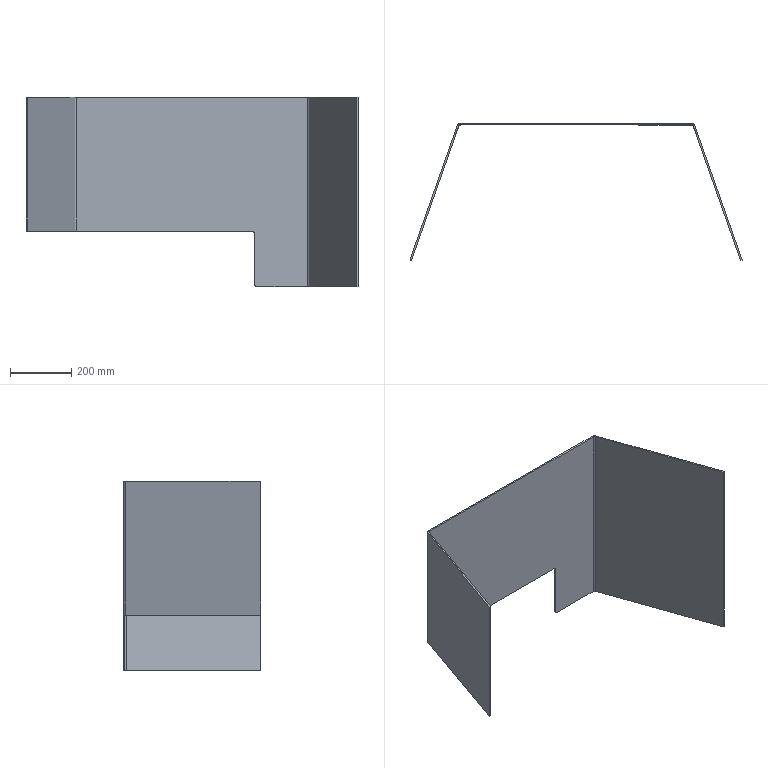Part | SolidWorks | features Fillet 2, Cut 1, FlatPattern 1, SMBaseFlange 1, SheetMetal 1, UnFold 1 | 1 solid | 24 faces | box 1088 x 449.658 x 620 mm | volume 4342657 mm3 | plane 18 | cylinder 6 | commonest cylinder face diameters 12 x2 22 x2 14 x1 20 x1
STEP:
#1=CARTESIAN_POINT('',(-378.607,0.,620.));
#2=VERTEX_POINT('',#1);
#3=CARTESIAN_POINT('',(-378.607,-5.,620.));
#4=VERTEX_POINT('',#3);
#5=CARTESIAN_POINT('',(-378.607,0.,620.));
#6=DIRECTION('',(0.,-1.,0.));
#7=VECTOR('',#6,1000.);
#8=LINE('',#5,#7);
#9=EDGE_CURVE('',#2,#4,#8,.T.);
#10=ORIENTED_EDGE('',*,*,#9,.F.);
#11=CARTESIAN_POINT('',(-388.985,-7.352,620.));
#12=VERTEX_POINT('',#11);
#13=CARTESIAN_POINT('',(-378.607,-11.,620.));
#14=DIRECTION('',(0.,0.,1.));
#15=DIRECTION('',(1.,0.,0.));
#16=AXIS2_PLACEMENT_3D('',#13,#14,#15);
#17=CIRCLE('',#16,11.);
#18=EDGE_CURVE('',#2,#12,#17,.T.);
#19=ORIENTED_EDGE('',*,*,#18,.T.);
#20=CARTESIAN_POINT('',(-384.268,-9.01,620.));
#21=VERTEX_POINT('',#20);
#22=CARTESIAN_POINT('',(-384.268,-9.01,620.));
#23=DIRECTION('',(-0.9434,0.3317,0.));
#24=VECTOR('',#23,1000.);
#25=LINE('',#22,#24);
#26=EDGE_CURVE('',#21,#12,#25,.T.);
#27=ORIENTED_EDGE('',*,*,#26,.F.);
#28=CARTESIAN_POINT('',(-378.607,-11.,620.));
#29=DIRECTION('',(0.,0.,1.));
#30=DIRECTION('',(1.,0.,0.));
#31=AXIS2_PLACEMENT_3D('',#28,#29,#30);
#32=CIRCLE('',#31,6.);
#33=EDGE_CURVE('',#4,#21,#32,.T.);
#34=ORIENTED_EDGE('',*,*,#33,.F.);
#35=EDGE_LOOP('',(#10,#19,#27,#34));
#36=FACE_OUTER_BOUND('',#35,.T.);
#37=CARTESIAN_POINT('',(-378.607,0.,620.));
#38=DIRECTION('',(0.,0.,1.));
#39=DIRECTION('',(1.,0.,0.));
#40=AXIS2_PLACEMENT_3D('',#37,#38,#39);
#41=PLANE('',#40);
#42=ADVANCED_FACE('',(#36),#41,.T.);
#43=CARTESIAN_POINT('',(378.607,0.,620.));
#44=VERTEX_POINT('',#43);
#45=CARTESIAN_POINT('',(-386.4,0.,620.));
#46=DIRECTION('',(-1.,0.,0.));
#47=VECTOR('',#46,1000.);
#48=LINE('',#45,#47);
#49=EDGE_CURVE('',#44,#2,#48,.T.);
#50=ORIENTED_EDGE('',*,*,#49,.T.);
#51=ORIENTED_EDGE('',*,*,#9,.T.);
#52=CARTESIAN_POINT('',(378.607,-5.,620.));
#53=VERTEX_POINT('',#52);
#54=CARTESIAN_POINT('',(-386.4,-5.,620.));
#55=DIRECTION('',(-1.,0.,0.));
#56=VECTOR('',#55,1000.);
#57=LINE('',#54,#56);
#58=EDGE_CURVE('',#53,#4,#57,.T.);
#59=ORIENTED_EDGE('',*,*,#58,.F.);
#60=CARTESIAN_POINT('',(378.607,-5.,620.));
#61=DIRECTION('',(0.,1.,0.));
#62=VECTOR('',#61,1000.);
#63=LINE('',#60,#62);
#64=EDGE_CURVE('',#53,#44,#63,.T.);
#65=ORIENTED_EDGE('',*,*,#64,.T.);
#66=EDGE_LOOP('',(#50,#51,#59,#65));
#67=FACE_OUTER_BOUND('',#66,.T.);
#68=CARTESIAN_POINT('',(-384.268,-9.01,620.));
#69=DIRECTION('',(0.,0.,1.));
#70=DIRECTION('',(1.,0.,0.));
#71=AXIS2_PLACEMENT_3D('',#68,#69,#70);
#72=PLANE('',#71);
#73=ADVANCED_FACE('',(#67),#72,.T.);
#74=CARTESIAN_POINT('',(388.985,-7.352,620.));
#75=VERTEX_POINT('',#74);
#76=CARTESIAN_POINT('',(384.268,-9.01,620.));
#77=VERTEX_POINT('',#76);
#78=CARTESIAN_POINT('',(388.985,-7.352,620.));
#79=DIRECTION('',(-0.9434,-0.3317,0.));
#80=VECTOR('',#79,1000.);
#81=LINE('',#78,#80);
#82=EDGE_CURVE('',#75,#77,#81,.T.);
#83=ORIENTED_EDGE('',*,*,#82,.F.);
#84=CARTESIAN_POINT('',(378.607,-11.,620.));
#85=DIRECTION('',(0.,0.,1.));
#86=DIRECTION('',(1.,0.,0.));
#87=AXIS2_PLACEMENT_3D('',#84,#85,#86);
#88=CIRCLE('',#87,11.);
#89=EDGE_CURVE('',#75,#44,#88,.T.);
#90=ORIENTED_EDGE('',*,*,#89,.T.);
#91=ORIENTED_EDGE('',*,*,#64,.F.);
#92=CARTESIAN_POINT('',(378.607,-11.,620.));
#93=DIRECTION('',(0.,0.,1.));
#94=DIRECTION('',(1.,0.,0.));
#95=AXIS2_PLACEMENT_3D('',#92,#93,#94);
#96=CIRCLE('',#95,6.);
#97=EDGE_CURVE('',#77,#53,#96,.T.);
#98=ORIENTED_EDGE('',*,*,#97,.F.);
#99=EDGE_LOOP('',(#83,#90,#91,#98));
#100=FACE_OUTER_BOUND('',#99,.T.);
#101=CARTESIAN_POINT('',(388.985,-7.352,620.));
#102=DIRECTION('',(0.,0.,1.));
#103=DIRECTION('',(1.,0.,0.));
#104=AXIS2_PLACEMENT_3D('',#101,#102,#103);
#105=PLANE('',#104);
#106=ADVANCED_FACE('',(#100),#105,.T.);
#107=CARTESIAN_POINT('',(543.902,-448.,620.));
#108=VERTEX_POINT('',#107);
#109=CARTESIAN_POINT('',(543.902,-448.,620.));
#110=DIRECTION('',(-0.3317,0.9434,0.));
#111=VECTOR('',#110,1000.);
#112=LINE('',#109,#111);
#113=EDGE_CURVE('',#108,#75,#112,.T.);
#114=ORIENTED_EDGE('',*,*,#113,.T.);
#115=ORIENTED_EDGE('',*,*,#82,.T.);
#116=CARTESIAN_POINT('',(539.185,-449.658,620.));
#117=VERTEX_POINT('',#116);
#118=CARTESIAN_POINT('',(539.185,-449.658,620.));
#119=DIRECTION('',(-0.3317,0.9434,0.));
#120=VECTOR('',#119,1000.);
#121=LINE('',#118,#120);
#122=EDGE_CURVE('',#117,#77,#121,.T.);
#123=ORIENTED_EDGE('',*,*,#122,.F.);
#124=CARTESIAN_POINT('',(543.902,-448.,620.));
#125=DIRECTION('',(-0.9434,-0.3317,0.));
#126=VECTOR('',#125,1000.);
#127=LINE('',#124,#126);
#128=EDGE_CURVE('',#108,#117,#127,.T.);
#129=ORIENTED_EDGE('',*,*,#128,.F.);
#130=EDGE_LOOP('',(#114,#115,#123,#129));
#131=FACE_OUTER_BOUND('',#130,.T.);
#132=CARTESIAN_POINT('',(378.607,-5.,620.));
#133=DIRECTION('',(0.,0.,1.));
#134=DIRECTION('',(1.,0.,0.));
#135=AXIS2_PLACEMENT_3D('',#132,#133,#134);
#136=PLANE('',#135);
#137=ADVANCED_FACE('',(#131),#136,.T.);
#138=CARTESIAN_POINT('',(378.607,0.,0.));
#139=VERTEX_POINT('',#138);
#140=CARTESIAN_POINT('',(378.607,-5.,0.));
#141=VERTEX_POINT('',#140);
#142=CARTESIAN_POINT('',(378.607,0.,0.));
#143=DIRECTION('',(0.,-1.,0.));
#144=VECTOR('',#143,1000.);
#145=LINE('',#142,#144);
#146=EDGE_CURVE('',#139,#141,#145,.T.);
#147=ORIENTED_EDGE('',*,*,#146,.F.);
#148=CARTESIAN_POINT('',(388.985,-7.352,0.));
#149=VERTEX_POINT('',#148);
#150=CARTESIAN_POINT('',(378.607,-11.,0.));
#151=DIRECTION('',(0.,0.,1.));
#152=DIRECTION('',(1.,0.,0.));
#153=AXIS2_PLACEMENT_3D('',#150,#151,#152);
#154=CIRCLE('',#153,11.);
#155=EDGE_CURVE('',#149,#139,#154,.T.);
#156=ORIENTED_EDGE('',*,*,#155,.F.);
#157=CARTESIAN_POINT('',(384.268,-9.01,0.));
#158=VERTEX_POINT('',#157);
#159=CARTESIAN_POINT('',(384.268,-9.01,0.));
#160=DIRECTION('',(0.9434,0.3317,0.));
#161=VECTOR('',#160,1000.);
#162=LINE('',#159,#161);
#163=EDGE_CURVE('',#158,#149,#162,.T.);
#164=ORIENTED_EDGE('',*,*,#163,.F.);
#165=CARTESIAN_POINT('',(378.607,-11.,0.));
#166=DIRECTION('',(0.,0.,1.));
#167=DIRECTION('',(1.,0.,0.));
#168=AXIS2_PLACEMENT_3D('',#165,#166,#167);
#169=CIRCLE('',#168,6.);
#170=EDGE_CURVE('',#158,#141,#169,.T.);
#171=ORIENTED_EDGE('',*,*,#170,.T.);
#172=EDGE_LOOP('',(#147,#156,#164,#171));
#173=FACE_OUTER_BOUND('',#172,.T.);
#174=CARTESIAN_POINT('',(378.607,0.,0.));
#175=DIRECTION('',(0.,0.,-1.));
#176=DIRECTION('',(-1.,0.,0.));
#177=AXIS2_PLACEMENT_3D('',#174,#175,#176);
#178=PLANE('',#177);
#179=ADVANCED_FACE('',(#173),#178,.T.);
#180=CARTESIAN_POINT('',(212.,-5.,0.));
#181=VERTEX_POINT('',#180);
#182=CARTESIAN_POINT('',(-386.4,-5.,0.));
#183=DIRECTION('',(-1.,0.,0.));
#184=VECTOR('',#183,1000.);
#185=LINE('',#182,#184);
#186=EDGE_CURVE('',#141,#181,#185,.T.);
#187=ORIENTED_EDGE('',*,*,#186,.T.);
#188=CARTESIAN_POINT('',(212.,0.,0.));
#189=VERTEX_POINT('',#188);
#190=CARTESIAN_POINT('',(212.,0.,0.));
#191=DIRECTION('',(0.,1.,0.));
#192=VECTOR('',#191,1000.);
#193=LINE('',#190,#192);
#194=EDGE_CURVE('',#181,#189,#193,.T.);
#195=ORIENTED_EDGE('',*,*,#194,.T.);
#196=CARTESIAN_POINT('',(-386.4,0.,0.));
#197=DIRECTION('',(-1.,0.,0.));
#198=VECTOR('',#197,1000.);
#199=LINE('',#196,#198);
#200=EDGE_CURVE('',#139,#189,#199,.T.);
#201=ORIENTED_EDGE('',*,*,#200,.F.);
#202=ORIENTED_EDGE('',*,*,#146,.T.);
#203=EDGE_LOOP('',(#187,#195,#201,#202));
#204=FACE_OUTER_BOUND('',#203,.T.);
#205=CARTESIAN_POINT('',(384.268,-9.01,0.));
#206=DIRECTION('',(0.,0.,-1.));
#207=DIRECTION('',(-1.,0.,0.));
#208=AXIS2_PLACEMENT_3D('',#205,#206,#207);
#209=PLANE('',#208);
#210=ADVANCED_FACE('',(#204),#209,.T.);
#211=CARTESIAN_POINT('',(-388.985,-7.352,182.));
#212=VERTEX_POINT('',#211);
#213=CARTESIAN_POINT('',(-388.985,-7.352,620.));
#214=DIRECTION('',(0.,0.,-1.));
#215=VECTOR('',#214,1000.);
#216=LINE('',#213,#215);
#217=EDGE_CURVE('',#12,#212,#216,.T.);
#218=ORIENTED_EDGE('',*,*,#217,.T.);
#219=CARTESIAN_POINT('',(-543.902,-448.,182.));
#220=VERTEX_POINT('',#219);
#221=CARTESIAN_POINT('',(-543.902,-448.,182.));
#222=DIRECTION('',(-0.3317,-0.9434,0.));
#223=VECTOR('',#222,1000.);
#224=LINE('',#221,#223);
#225=EDGE_CURVE('',#212,#220,#224,.T.);
#226=ORIENTED_EDGE('',*,*,#225,.T.);
#227=CARTESIAN_POINT('',(-543.902,-448.,620.));
#228=VERTEX_POINT('',#227);
#229=CARTESIAN_POINT('',(-543.902,-448.,620.));
#230=DIRECTION('',(0.,0.,-1.));
#231=VECTOR('',#230,1000.);
#232=LINE('',#229,#231);
#233=EDGE_CURVE('',#228,#220,#232,.T.);
#234=ORIENTED_EDGE('',*,*,#233,.F.);
#235=CARTESIAN_POINT('',(-543.902,-448.,620.));
#236=DIRECTION('',(-0.3317,-0.9434,0.));
#237=VECTOR('',#236,1000.);
#238=LINE('',#235,#237);
#239=EDGE_CURVE('',#12,#228,#238,.T.);
#240=ORIENTED_EDGE('',*,*,#239,.F.);
#241=EDGE_LOOP('',(#218,#226,#234,#240));
#242=FACE_OUTER_BOUND('',#241,.T.);
#243=CARTESIAN_POINT('',(-543.902,-448.,620.));
#244=DIRECTION('',(0.9434,-0.3317,0.));
#245=DIRECTION('',(0.3317,0.9434,0.));
#246=AXIS2_PLACEMENT_3D('',#243,#244,#245);
#247=PLANE('',#246);
#248=ADVANCED_FACE('',(#242),#247,.F.);
#249=CARTESIAN_POINT('',(-539.185,-449.658,182.));
#250=VERTEX_POINT('',#249);
#251=CARTESIAN_POINT('',(-539.185,-449.658,182.));
#252=DIRECTION('',(-0.9434,0.3317,0.));
#253=VECTOR('',#252,1000.);
#254=LINE('',#251,#253);
#255=EDGE_CURVE('',#250,#220,#254,.T.);
#256=ORIENTED_EDGE('',*,*,#255,.F.);
#257=CARTESIAN_POINT('',(-539.185,-449.658,620.));
#258=VERTEX_POINT('',#257);
#259=CARTESIAN_POINT('',(-539.185,-449.658,620.));
#260=DIRECTION('',(0.,0.,-1.));
#261=VECTOR('',#260,1000.);
#262=LINE('',#259,#261);
#263=EDGE_CURVE('',#258,#250,#262,.T.);
#264=ORIENTED_EDGE('',*,*,#263,.F.);
#265=CARTESIAN_POINT('',(-539.185,-449.658,620.));
#266=DIRECTION('',(-0.9434,0.3317,0.));
#267=VECTOR('',#266,1000.);
#268=LINE('',#265,#267);
#269=EDGE_CURVE('',#258,#228,#268,.T.);
#270=ORIENTED_EDGE('',*,*,#269,.T.);
#271=ORIENTED_EDGE('',*,*,#233,.T.);
#272=EDGE_LOOP('',(#256,#264,#270,#271));
#273=FACE_OUTER_BOUND('',#272,.T.);
#274=CARTESIAN_POINT('',(-539.185,-449.658,620.));
#275=DIRECTION('',(-0.3317,-0.9434,0.));
#276=DIRECTION('',(0.9434,-0.3317,0.));
#277=AXIS2_PLACEMENT_3D('',#274,#275,#276);
#278=PLANE('',#277);
#279=ADVANCED_FACE('',(#273),#278,.T.);
#280=CARTESIAN_POINT('',(-384.268,-9.01,182.));
#281=VERTEX_POINT('',#280);
#282=CARTESIAN_POINT('',(-539.185,-449.658,182.));
#283=DIRECTION('',(-0.3317,-0.9434,0.));
#284=VECTOR('',#283,1000.);
#285=LINE('',#282,#284);
#286=EDGE_CURVE('',#281,#250,#285,.T.);
#287=ORIENTED_EDGE('',*,*,#286,.F.);
#288=CARTESIAN_POINT('',(-384.268,-9.01,620.));
#289=DIRECTION('',(0.,0.,-1.));
#290=VECTOR('',#289,1000.);
#291=LINE('',#288,#290);
#292=EDGE_CURVE('',#21,#281,#291,.T.);
#293=ORIENTED_EDGE('',*,*,#292,.F.);
#294=CARTESIAN_POINT('',(-539.185,-449.658,620.));
#295=DIRECTION('',(-0.3317,-0.9434,0.));
#296=VECTOR('',#295,1000.);
#297=LINE('',#294,#296);
#298=EDGE_CURVE('',#21,#258,#297,.T.);
#299=ORIENTED_EDGE('',*,*,#298,.T.);
#300=ORIENTED_EDGE('',*,*,#263,.T.);
#301=EDGE_LOOP('',(#287,#293,#299,#300));
#302=FACE_OUTER_BOUND('',#301,.T.);
#303=CARTESIAN_POINT('',(-539.185,-449.658,620.));
#304=DIRECTION('',(0.9434,-0.3317,0.));
#305=DIRECTION('',(0.3317,0.9434,0.));
#306=AXIS2_PLACEMENT_3D('',#303,#304,#305);
#307=PLANE('',#306);
#308=ADVANCED_FACE('',(#302),#307,.T.);
#309=CARTESIAN_POINT('',(-378.607,-5.,182.));
#310=VERTEX_POINT('',#309);
#311=CARTESIAN_POINT('',(-378.607,-11.,182.));
#312=DIRECTION('',(0.,0.,1.));
#313=DIRECTION('',(1.,0.,0.));
#314=AXIS2_PLACEMENT_3D('',#311,#312,#313);
#315=CIRCLE('',#314,6.);
#316=EDGE_CURVE('',#310,#281,#315,.T.);
#317=ORIENTED_EDGE('',*,*,#316,.F.);
#318=CARTESIAN_POINT('',(-378.607,-5.,620.));
#319=DIRECTION('',(0.,0.,-1.));
#320=VECTOR('',#319,1000.);
#321=LINE('',#318,#320);
#322=EDGE_CURVE('',#4,#310,#321,.T.);
#323=ORIENTED_EDGE('',*,*,#322,.F.);
#324=ORIENTED_EDGE('',*,*,#33,.T.);
#325=ORIENTED_EDGE('',*,*,#292,.T.);
#326=EDGE_LOOP('',(#317,#323,#324,#325));
#327=FACE_OUTER_BOUND('',#326,.T.);
#328=CARTESIAN_POINT('',(-378.607,-11.,620.));
#329=DIRECTION('',(0.,0.,-1.));
#330=DIRECTION('',(-1.,0.,0.));
#331=AXIS2_PLACEMENT_3D('',#328,#329,#330);
#332=CYLINDRICAL_SURFACE('',#331,6.);
#333=ADVANCED_FACE('',(#327),#332,.F.);
#334=CARTESIAN_POINT('',(205.,-5.,7.));
#335=VERTEX_POINT('',#334);
#336=CARTESIAN_POINT('',(205.,-5.,172.));
#337=VERTEX_POINT('',#336);
#338=CARTESIAN_POINT('',(205.,-5.,620.));
#339=DIRECTION('',(0.,0.,1.));
#340=VECTOR('',#339,1000.);
#341=LINE('',#338,#340);
#342=EDGE_CURVE('',#335,#337,#341,.T.);
#343=ORIENTED_EDGE('',*,*,#342,.F.);
#344=CARTESIAN_POINT('',(212.,-5.,7.));
#345=DIRECTION('',(0.,-1.,0.));
#346=DIRECTION('',(1.,0.,0.));
#347=AXIS2_PLACEMENT_3D('',#344,#345,#346);
#348=CIRCLE('',#347,7.);
#349=EDGE_CURVE('',#335,#181,#348,.T.);
#350=ORIENTED_EDGE('',*,*,#349,.T.);
#351=ORIENTED_EDGE('',*,*,#186,.F.);
#352=CARTESIAN_POINT('',(378.607,-5.,620.));
#353=DIRECTION('',(0.,0.,-1.));
#354=VECTOR('',#353,1000.);
#355=LINE('',#352,#354);
#356=EDGE_CURVE('',#53,#141,#355,.T.);
#357=ORIENTED_EDGE('',*,*,#356,.F.);
#358=ORIENTED_EDGE('',*,*,#58,.T.);
#359=ORIENTED_EDGE('',*,*,#322,.T.);
#360=CARTESIAN_POINT('',(195.,-5.,182.));
#361=VERTEX_POINT('',#360);
#362=CARTESIAN_POINT('',(-386.4,-5.,182.));
#363=DIRECTION('',(-1.,0.,0.));
#364=VECTOR('',#363,1000.);
#365=LINE('',#362,#364);
#366=EDGE_CURVE('',#361,#310,#365,.T.);
#367=ORIENTED_EDGE('',*,*,#366,.F.);
#368=CARTESIAN_POINT('',(195.,-5.,172.));
#369=DIRECTION('',(0.,1.,0.));
#370=DIRECTION('',(1.,0.,0.));
#371=AXIS2_PLACEMENT_3D('',#368,#369,#370);
#372=CIRCLE('',#371,10.);
#373=EDGE_CURVE('',#361,#337,#372,.T.);
#374=ORIENTED_EDGE('',*,*,#373,.T.);
#375=EDGE_LOOP('',(#343,#350,#351,#357,#358,#359,#367,#374));
#376=FACE_OUTER_BOUND('',#375,.T.);
#377=CARTESIAN_POINT('',(-386.4,-5.,620.));
#378=DIRECTION('',(0.,-1.,0.));
#379=DIRECTION('',(1.,0.,0.));
#380=AXIS2_PLACEMENT_3D('',#377,#378,#379);
#381=PLANE('',#380);
#382=ADVANCED_FACE('',(#376),#381,.T.);
#383=ORIENTED_EDGE('',*,*,#170,.F.);
#384=CARTESIAN_POINT('',(384.268,-9.01,620.));
#385=DIRECTION('',(0.,0.,-1.));
#386=VECTOR('',#385,1000.);
#387=LINE('',#384,#386);
#388=EDGE_CURVE('',#77,#158,#387,.T.);
#389=ORIENTED_EDGE('',*,*,#388,.F.);
#390=ORIENTED_EDGE('',*,*,#97,.T.);
#391=ORIENTED_EDGE('',*,*,#356,.T.);
#392=EDGE_LOOP('',(#383,#389,#390,#391));
#393=FACE_OUTER_BOUND('',#392,.T.);
#394=CARTESIAN_POINT('',(378.607,-11.,620.));
#395=DIRECTION('',(0.,0.,-1.));
#396=DIRECTION('',(-1.,0.,0.));
#397=AXIS2_PLACEMENT_3D('',#394,#395,#396);
#398=CYLINDRICAL_SURFACE('',#397,6.);
#399=ADVANCED_FACE('',(#393),#398,.F.);
#400=CARTESIAN_POINT('',(539.185,-449.658,0.));
#401=VERTEX_POINT('',#400);
#402=CARTESIAN_POINT('',(539.185,-449.658,0.));
#403=DIRECTION('',(-0.3317,0.9434,0.));
#404=VECTOR('',#403,1000.);
#405=LINE('',#402,#404);
#406=EDGE_CURVE('',#401,#158,#405,.T.);
#407=ORIENTED_EDGE('',*,*,#406,.F.);
#408=CARTESIAN_POINT('',(539.185,-449.658,620.));
#409=DIRECTION('',(0.,0.,-1.));
#410=VECTOR('',#409,1000.);
#411=LINE('',#408,#410);
#412=EDGE_CURVE('',#117,#401,#411,.T.);
#413=ORIENTED_EDGE('',*,*,#412,.F.);
#414=ORIENTED_EDGE('',*,*,#122,.T.);
#415=ORIENTED_EDGE('',*,*,#388,.T.);
#416=EDGE_LOOP('',(#407,#413,#414,#415));
#417=FACE_OUTER_BOUND('',#416,.T.);
#418=CARTESIAN_POINT('',(539.185,-449.658,620.));
#419=DIRECTION('',(-0.9434,-0.3317,0.));
#420=DIRECTION('',(0.3317,-0.9434,0.));
#421=AXIS2_PLACEMENT_3D('',#418,#419,#420);
#422=PLANE('',#421);
#423=ADVANCED_FACE('',(#417),#422,.T.);
#424=CARTESIAN_POINT('',(543.902,-448.,0.));
#425=VERTEX_POINT('',#424);
#426=CARTESIAN_POINT('',(543.902,-448.,0.));
#427=DIRECTION('',(-0.9434,-0.3317,0.));
#428=VECTOR('',#427,1000.);
#429=LINE('',#426,#428);
#430=EDGE_CURVE('',#425,#401,#429,.T.);
#431=ORIENTED_EDGE('',*,*,#430,.F.);
#432=CARTESIAN_POINT('',(543.902,-448.,620.));
#433=DIRECTION('',(0.,0.,-1.));
#434=VECTOR('',#433,1000.);
#435=LINE('',#432,#434);
#436=EDGE_CURVE('',#108,#425,#435,.T.);
#437=ORIENTED_EDGE('',*,*,#436,.F.);
#438=ORIENTED_EDGE('',*,*,#128,.T.);
#439=ORIENTED_EDGE('',*,*,#412,.T.);
#440=EDGE_LOOP('',(#431,#437,#438,#439));
#441=FACE_OUTER_BOUND('',#440,.T.);
#442=CARTESIAN_POINT('',(543.902,-448.,620.));
#443=DIRECTION('',(0.3317,-0.9434,0.));
#444=DIRECTION('',(0.9434,0.3317,0.));
#445=AXIS2_PLACEMENT_3D('',#442,#443,#444);
#446=PLANE('',#445);
#447=ADVANCED_FACE('',(#441),#446,.T.);
#448=CARTESIAN_POINT('',(543.902,-448.,0.));
#449=DIRECTION('',(-0.3317,0.9434,0.));
#450=VECTOR('',#449,1000.);
#451=LINE('',#448,#450);
#452=EDGE_CURVE('',#425,#149,#451,.T.);
#453=ORIENTED_EDGE('',*,*,#452,.T.);
#454=CARTESIAN_POINT('',(388.985,-7.352,620.));
#455=DIRECTION('',(0.,0.,-1.));
#456=VECTOR('',#455,1000.);
#457=LINE('',#454,#456);
#458=EDGE_CURVE('',#75,#149,#457,.T.);
#459=ORIENTED_EDGE('',*,*,#458,.F.);
#460=ORIENTED_EDGE('',*,*,#113,.F.);
#461=ORIENTED_EDGE('',*,*,#436,.T.);
#462=EDGE_LOOP('',(#453,#459,#460,#461));
#463=FACE_OUTER_BOUND('',#462,.T.);
#464=CARTESIAN_POINT('',(543.902,-448.,620.));
#465=DIRECTION('',(-0.9434,-0.3317,0.));
#466=DIRECTION('',(0.3317,-0.9434,0.));
#467=AXIS2_PLACEMENT_3D('',#464,#465,#466);
#468=PLANE('',#467);
#469=ADVANCED_FACE('',(#463),#468,.F.);
#470=ORIENTED_EDGE('',*,*,#155,.T.);
#471=CARTESIAN_POINT('',(378.607,0.,620.));
#472=DIRECTION('',(0.,0.,-1.));
#473=VECTOR('',#472,1000.);
#474=LINE('',#471,#473);
#475=EDGE_CURVE('',#44,#139,#474,.T.);
#476=ORIENTED_EDGE('',*,*,#475,.F.);
#477=ORIENTED_EDGE('',*,*,#89,.F.);
#478=ORIENTED_EDGE('',*,*,#458,.T.);
#479=EDGE_LOOP('',(#470,#476,#477,#478));
#480=FACE_OUTER_BOUND('',#479,.T.);
#481=CARTESIAN_POINT('',(378.607,-11.,620.));
#482=DIRECTION('',(0.,0.,-1.));
#483=DIRECTION('',(-1.,0.,0.));
#484=AXIS2_PLACEMENT_3D('',#481,#482,#483);
#485=CYLINDRICAL_SURFACE('',#484,11.);
#486=ADVANCED_FACE('',(#480),#485,.T.);
#487=ORIENTED_EDGE('',*,*,#200,.T.);
#488=CARTESIAN_POINT('',(205.,0.,7.));
#489=VERTEX_POINT('',#488);
#490=CARTESIAN_POINT('',(212.,0.,7.));
#491=DIRECTION('',(0.,1.,0.));
#492=DIRECTION('',(1.,0.,0.));
#493=AXIS2_PLACEMENT_3D('',#490,#491,#492);
#494=CIRCLE('',#493,7.);
#495=EDGE_CURVE('',#189,#489,#494,.T.);
#496=ORIENTED_EDGE('',*,*,#495,.T.);
#497=CARTESIAN_POINT('',(205.,0.,172.));
#498=VERTEX_POINT('',#497);
#499=CARTESIAN_POINT('',(205.,0.,620.));
#500=DIRECTION('',(0.,0.,1.));
#501=VECTOR('',#500,1000.);
#502=LINE('',#499,#501);
#503=EDGE_CURVE('',#489,#498,#502,.T.);
#504=ORIENTED_EDGE('',*,*,#503,.T.);
#505=CARTESIAN_POINT('',(195.,0.,182.));
#506=VERTEX_POINT('',#505);
#507=CARTESIAN_POINT('',(195.,0.,172.));
#508=DIRECTION('',(0.,-1.,0.));
#509=DIRECTION('',(1.,0.,0.));
#510=AXIS2_PLACEMENT_3D('',#507,#508,#509);
#511=CIRCLE('',#510,10.);
#512=EDGE_CURVE('',#498,#506,#511,.T.);
#513=ORIENTED_EDGE('',*,*,#512,.T.);
#514=CARTESIAN_POINT('',(-378.607,0.,182.));
#515=VERTEX_POINT('',#514);
#516=CARTESIAN_POINT('',(-386.4,0.,182.));
#517=DIRECTION('',(-1.,0.,0.));
#518=VECTOR('',#517,1000.);
#519=LINE('',#516,#518);
#520=EDGE_CURVE('',#506,#515,#519,.T.);
#521=ORIENTED_EDGE('',*,*,#520,.T.);
#522=CARTESIAN_POINT('',(-378.607,0.,620.));
#523=DIRECTION('',(0.,0.,-1.));
#524=VECTOR('',#523,1000.);
#525=LINE('',#522,#524);
#526=EDGE_CURVE('',#2,#515,#525,.T.);
#527=ORIENTED_EDGE('',*,*,#526,.F.);
#528=ORIENTED_EDGE('',*,*,#49,.F.);
#529=ORIENTED_EDGE('',*,*,#475,.T.);
#530=EDGE_LOOP('',(#487,#496,#504,#513,#521,#527,#528,#529));
#531=FACE_OUTER_BOUND('',#530,.T.);
#532=CARTESIAN_POINT('',(-386.4,0.,620.));
#533=DIRECTION('',(0.,-1.,0.));
#534=DIRECTION('',(1.,0.,0.));
#535=AXIS2_PLACEMENT_3D('',#532,#533,#534);
#536=PLANE('',#535);
#537=ADVANCED_FACE('',(#531),#536,.F.);
#538=ORIENTED_EDGE('',*,*,#526,.T.);
#539=CARTESIAN_POINT('',(-378.607,-11.,182.));
#540=DIRECTION('',(0.,0.,1.));
#541=DIRECTION('',(1.,0.,0.));
#542=AXIS2_PLACEMENT_3D('',#539,#540,#541);
#543=CIRCLE('',#542,11.);
#544=EDGE_CURVE('',#515,#212,#543,.T.);
#545=ORIENTED_EDGE('',*,*,#544,.T.);
#546=ORIENTED_EDGE('',*,*,#217,.F.);
#547=ORIENTED_EDGE('',*,*,#18,.F.);
#548=EDGE_LOOP('',(#538,#545,#546,#547));
#549=FACE_OUTER_BOUND('',#548,.T.);
#550=CARTESIAN_POINT('',(-378.607,-11.,620.));
#551=DIRECTION('',(0.,0.,-1.));
#552=DIRECTION('',(-1.,0.,0.));
#553=AXIS2_PLACEMENT_3D('',#550,#551,#552);
#554=CYLINDRICAL_SURFACE('',#553,11.);
#555=ADVANCED_FACE('',(#549),#554,.T.);
#556=ORIENTED_EDGE('',*,*,#239,.T.);
#557=ORIENTED_EDGE('',*,*,#269,.F.);
#558=ORIENTED_EDGE('',*,*,#298,.F.);
#559=ORIENTED_EDGE('',*,*,#26,.T.);
#560=EDGE_LOOP('',(#556,#557,#558,#559));
#561=FACE_OUTER_BOUND('',#560,.T.);
#562=CARTESIAN_POINT('',(-378.607,-11.,620.));
#563=DIRECTION('',(0.,0.,1.));
#564=DIRECTION('',(1.,0.,0.));
#565=AXIS2_PLACEMENT_3D('',#562,#563,#564);
#566=PLANE('',#565);
#567=ADVANCED_FACE('',(#561),#566,.T.);
#568=ORIENTED_EDGE('',*,*,#406,.T.);
#569=ORIENTED_EDGE('',*,*,#163,.T.);
#570=ORIENTED_EDGE('',*,*,#452,.F.);
#571=ORIENTED_EDGE('',*,*,#430,.T.);
#572=EDGE_LOOP('',(#568,#569,#570,#571));
#573=FACE_OUTER_BOUND('',#572,.T.);
#574=CARTESIAN_POINT('',(-378.607,-11.,0.));
#575=DIRECTION('',(0.,0.,1.));
#576=DIRECTION('',(1.,0.,0.));
#577=AXIS2_PLACEMENT_3D('',#574,#575,#576);
#578=PLANE('',#577);
#579=ADVANCED_FACE('',(#573),#578,.F.);
#580=ORIENTED_EDGE('',*,*,#342,.T.);
#581=CARTESIAN_POINT('',(205.,0.,172.));
#582=DIRECTION('',(0.,1.,0.));
#583=VECTOR('',#582,1000.);
#584=LINE('',#581,#583);
#585=EDGE_CURVE('',#337,#498,#584,.T.);
#586=ORIENTED_EDGE('',*,*,#585,.T.);
#587=ORIENTED_EDGE('',*,*,#503,.F.);
#588=CARTESIAN_POINT('',(205.,-5.,7.));
#589=DIRECTION('',(0.,-1.,0.));
#590=VECTOR('',#589,1000.);
#591=LINE('',#588,#590);
#592=EDGE_CURVE('',#489,#335,#591,.T.);
#593=ORIENTED_EDGE('',*,*,#592,.T.);
#594=EDGE_LOOP('',(#580,#586,#587,#593));
#595=FACE_OUTER_BOUND('',#594,.T.);
#596=CARTESIAN_POINT('',(205.,-449.658,-60.503));
#597=DIRECTION('',(1.,0.,0.));
#598=DIRECTION('',(0.,0.,-1.));
#599=AXIS2_PLACEMENT_3D('',#596,#597,#598);
#600=PLANE('',#599);
#601=ADVANCED_FACE('',(#595),#600,.F.);
#602=ORIENTED_EDGE('',*,*,#520,.F.);
#603=CARTESIAN_POINT('',(195.,-5.,182.));
#604=DIRECTION('',(0.,-1.,0.));
#605=VECTOR('',#604,1000.);
#606=LINE('',#603,#605);
#607=EDGE_CURVE('',#506,#361,#606,.T.);
#608=ORIENTED_EDGE('',*,*,#607,.T.);
#609=ORIENTED_EDGE('',*,*,#366,.T.);
#610=ORIENTED_EDGE('',*,*,#316,.T.);
#611=ORIENTED_EDGE('',*,*,#286,.T.);
#612=ORIENTED_EDGE('',*,*,#255,.T.);
#613=ORIENTED_EDGE('',*,*,#225,.F.);
#614=ORIENTED_EDGE('',*,*,#544,.F.);
#615=EDGE_LOOP('',(#602,#608,#609,#610,#611,#612,#613,#614));
#616=FACE_OUTER_BOUND('',#615,.T.);
#617=CARTESIAN_POINT('',(-661.016,-449.658,182.));
#618=DIRECTION('',(0.,0.,1.));
#619=DIRECTION('',(1.,0.,0.));
#620=AXIS2_PLACEMENT_3D('',#617,#618,#619);
#621=PLANE('',#620);
#622=ADVANCED_FACE('',(#616),#621,.F.);
#623=ORIENTED_EDGE('',*,*,#495,.F.);
#624=ORIENTED_EDGE('',*,*,#194,.F.);
#625=ORIENTED_EDGE('',*,*,#349,.F.);
#626=ORIENTED_EDGE('',*,*,#592,.F.);
#627=EDGE_LOOP('',(#623,#624,#625,#626));
#628=FACE_OUTER_BOUND('',#627,.T.);
#629=CARTESIAN_POINT('',(212.,-449.658,7.));
#630=DIRECTION('',(0.,1.,0.));
#631=DIRECTION('',(0.,0.,1.));
#632=AXIS2_PLACEMENT_3D('',#629,#630,#631);
#633=CYLINDRICAL_SURFACE('',#632,7.);
#634=ADVANCED_FACE('',(#628),#633,.T.);
#635=ORIENTED_EDGE('',*,*,#373,.F.);
#636=ORIENTED_EDGE('',*,*,#607,.F.);
#637=ORIENTED_EDGE('',*,*,#512,.F.);
#638=ORIENTED_EDGE('',*,*,#585,.F.);
#639=EDGE_LOOP('',(#635,#636,#637,#638));
#640=FACE_OUTER_BOUND('',#639,.T.);
#641=CARTESIAN_POINT('',(195.,-449.658,172.));
#642=DIRECTION('',(0.,-1.,0.));
#643=DIRECTION('',(0.,0.,-1.));
#644=AXIS2_PLACEMENT_3D('',#641,#642,#643);
#645=CYLINDRICAL_SURFACE('',#644,10.);
#646=ADVANCED_FACE('',(#640),#645,.F.);
#647=CLOSED_SHELL('',(#42,#73,#106,#137,#179,#210,#248,#279,#308,#333,#382,#399,#423,#447,#469,#486,#537,#555,#567,#579,#601,#622,#634,#646));
#648=MANIFOLD_SOLID_BREP('',#647);
#649=CARTESIAN_POINT('',(0.,0.,0.));
#650=DIRECTION('',(0.,0.,1.));
#651=DIRECTION('',(1.,0.,0.));
#652=AXIS2_PLACEMENT_3D('',#649,#650,#651);
#653=(LENGTH_UNIT()NAMED_UNIT(*)SI_UNIT(.MILLI.,.METRE.));
#654=UNCERTAINTY_MEASURE_WITH_UNIT(LENGTH_MEASURE(0.00001),#653,'','');
#655=(NAMED_UNIT(*)PLANE_ANGLE_UNIT()SI_UNIT($,.RADIAN.));
#656=(NAMED_UNIT(*)SI_UNIT($,.STERADIAN.)SOLID_ANGLE_UNIT());
#657=(GEOMETRIC_REPRESENTATION_CONTEXT(3)GLOBAL_UNCERTAINTY_ASSIGNED_CONTEXT((#654))GLOBAL_UNIT_ASSIGNED_CONTEXT((#653,#655,#656))REPRESENTATION_CONTEXT('',''));
#658=ADVANCED_BREP_SHAPE_REPRESENTATION('',(#648,#652),#657);